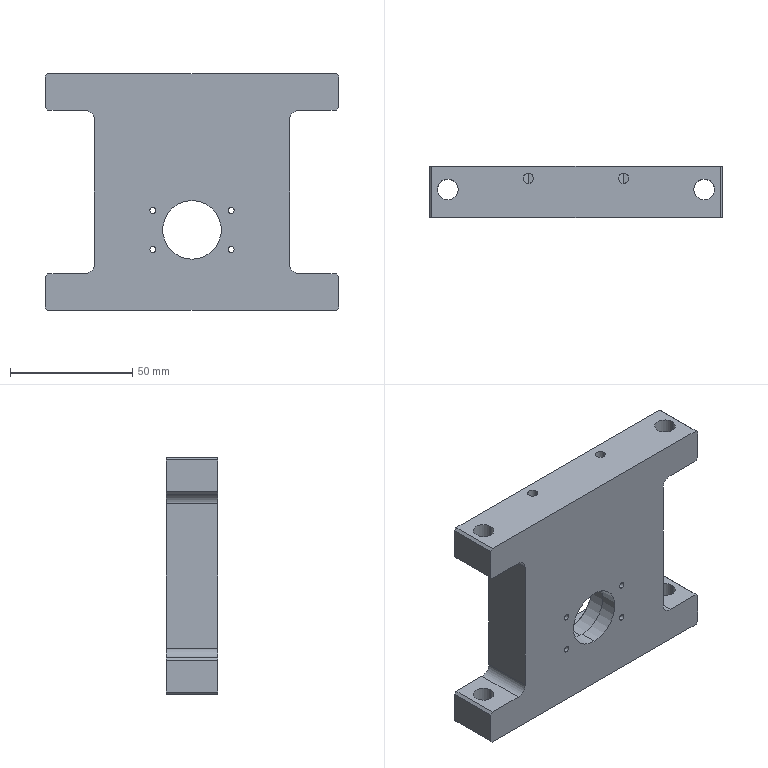Part | STEP file | PN_0001 Front Guide Channel Support Plate Left | 1 solid | 72 faces | box 120 x 21 x 97 mm | volume 164899 mm3 | cylinder 36 | plane 30 | cone 6 | commonest cylinder face diameters 2.5 x8 8.5 x8 4 x4 4.2 x4 8 x4 16 x4